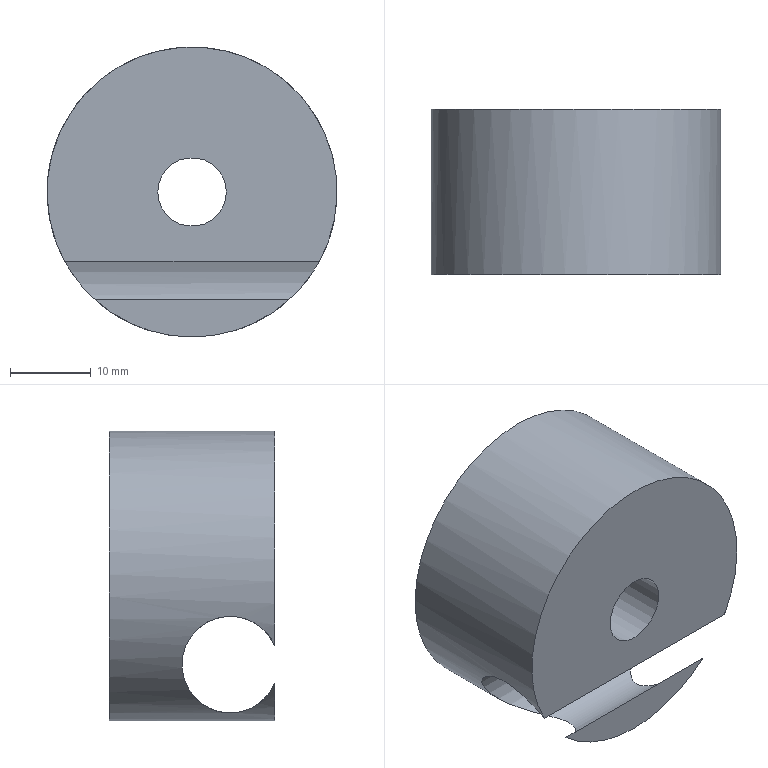Part | STEP file | 冲床-300配套压波_id454_x_t | 1 solid | 8 faces | box 36 x 20.5 x 36 mm | volume 15877 mm3 | cylinder 4 | plane 4 | commonest cylinder face diameters 8.5 x1 12 x1 14 x1 36 x1
STEP:
#1=CARTESIAN_POINT('',(1126.,-87.,-85.));
#2=VERTEX_POINT('',#1);
#3=CARTESIAN_POINT('',(1126.,-87.,-103.));
#4=DIRECTION('',(0.,-1.,0.));
#5=DIRECTION('',(0.,0.,1.));
#6=AXIS2_PLACEMENT_3D('',#3,#4,#5);
#7=CIRCLE('',#6,18.);
#8=EDGE_CURVE('',#2,#2,#7,.T.);
#9=ORIENTED_EDGE('',*,*,#8,.T.);
#10=EDGE_LOOP('',(#9));
#11=FACE_BOUND('',#10,.T.);
#12=CARTESIAN_POINT('',(1141.812,-107.5,-111.602));
#13=VERTEX_POINT('',#12);
#14=CARTESIAN_POINT('',(1110.188,-107.5,-111.602));
#15=VERTEX_POINT('',#14);
#16=CARTESIAN_POINT('',(1126.,-107.5,-103.));
#17=DIRECTION('',(0.,-1.,0.));
#18=DIRECTION('',(1.,0.,0.));
#19=AXIS2_PLACEMENT_3D('',#16,#17,#18);
#20=CIRCLE('',#19,18.);
#21=EDGE_CURVE('',#13,#15,#20,.T.);
#22=ORIENTED_EDGE('',*,*,#21,.F.);
#23=CARTESIAN_POINT('',(1138.021,-107.5,-116.398));
#24=VERTEX_POINT('',#23);
#25=CARTESIAN_POINT('',(1141.812,-107.5,-111.602));
#26=CARTESIAN_POINT('',(1142.553,-106.906,-110.24));
#27=CARTESIAN_POINT('',(1142.98,-105.701,-109.004));
#28=CARTESIAN_POINT('',(1143.354,-102.667,-107.819));
#29=CARTESIAN_POINT('',(1143.342,-100.878,-107.881));
#30=CARTESIAN_POINT('',(1142.876,-97.917,-109.307));
#31=CARTESIAN_POINT('',(1142.38,-96.833,-110.626));
#32=CARTESIAN_POINT('',(1140.814,-95.864,-113.345));
#33=CARTESIAN_POINT('',(1139.756,-95.929,-114.718));
#34=CARTESIAN_POINT('',(1137.484,-96.646,-116.952));
#35=CARTESIAN_POINT('',(1136.238,-97.289,-117.872));
#36=CARTESIAN_POINT('',(1134.415,-98.534,-118.928));
#37=CARTESIAN_POINT('',(1133.8,-99.005,-119.234));
#38=CARTESIAN_POINT('',(1132.684,-100.104,-119.724));
#39=CARTESIAN_POINT('',(1132.126,-100.766,-119.926));
#40=CARTESIAN_POINT('',(1131.796,-102.369,-120.042));
#41=CARTESIAN_POINT('',(1132.18,-103.204,-119.914));
#42=CARTESIAN_POINT('',(1133.181,-104.454,-119.514));
#43=CARTESIAN_POINT('',(1133.782,-104.966,-119.245));
#44=CARTESIAN_POINT('',(1135.59,-106.337,-118.293));
#45=CARTESIAN_POINT('',(1136.839,-107.038,-117.458));
#46=CARTESIAN_POINT('',(1138.021,-107.5,-116.398));
#47=B_SPLINE_CURVE_WITH_KNOTS('',3,(#25,#26,#27,#28,#29,#30,#31,#32,#33,#34,#35,#36,#37,#38,#39,#40,#41,#42,#43,#44,#45,#46),.UNSPECIFIED.,.F.,.F.,(4,2,2,2,2,2,2,2,2,2,4),(0.,0.125,0.25,0.375,0.5,0.625,0.6875,0.75,0.8125,0.875,1.),.UNSPECIFIED.);
#48=EDGE_CURVE('',#13,#24,#47,.T.);
#49=ORIENTED_EDGE('',*,*,#48,.T.);
#50=CARTESIAN_POINT('',(1113.979,-107.5,-116.398));
#51=VERTEX_POINT('',#50);
#52=CARTESIAN_POINT('',(1126.,-107.5,-103.));
#53=DIRECTION('',(0.,-1.,0.));
#54=DIRECTION('',(1.,0.,0.));
#55=AXIS2_PLACEMENT_3D('',#52,#53,#54);
#56=CIRCLE('',#55,18.);
#57=EDGE_CURVE('',#51,#24,#56,.T.);
#58=ORIENTED_EDGE('',*,*,#57,.F.);
#59=CARTESIAN_POINT('',(1113.979,-107.5,-116.398));
#60=CARTESIAN_POINT('',(1115.162,-107.037,-117.459));
#61=CARTESIAN_POINT('',(1116.404,-106.341,-118.29));
#62=CARTESIAN_POINT('',(1118.222,-104.963,-119.247));
#63=CARTESIAN_POINT('',(1118.822,-104.45,-119.516));
#64=CARTESIAN_POINT('',(1119.819,-103.205,-119.914));
#65=CARTESIAN_POINT('',(1120.205,-102.374,-120.043));
#66=CARTESIAN_POINT('',(1119.873,-100.76,-119.926));
#67=CARTESIAN_POINT('',(1119.316,-100.104,-119.724));
#68=CARTESIAN_POINT('',(1118.201,-99.005,-119.234));
#69=CARTESIAN_POINT('',(1117.586,-98.534,-118.928));
#70=CARTESIAN_POINT('',(1115.76,-97.287,-117.87));
#71=CARTESIAN_POINT('',(1114.517,-96.646,-116.953));
#72=CARTESIAN_POINT('',(1112.244,-95.929,-114.718));
#73=CARTESIAN_POINT('',(1111.191,-95.863,-113.353));
#74=CARTESIAN_POINT('',(1109.621,-96.83,-110.63));
#75=CARTESIAN_POINT('',(1109.125,-97.923,-109.309));
#76=CARTESIAN_POINT('',(1108.662,-100.843,-107.893));
#77=CARTESIAN_POINT('',(1108.644,-102.64,-107.812));
#78=CARTESIAN_POINT('',(1109.019,-105.707,-109.004));
#79=CARTESIAN_POINT('',(1109.446,-106.905,-110.238));
#80=CARTESIAN_POINT('',(1110.188,-107.5,-111.602));
#81=B_SPLINE_CURVE_WITH_KNOTS('',3,(#59,#60,#61,#62,#63,#64,#65,#66,#67,#68,#69,#70,#71,#72,#73,#74,#75,#76,#77,#78,#79,#80),.UNSPECIFIED.,.F.,.F.,(4,2,2,2,2,2,2,2,2,2,4),(0.,0.125,0.1875,0.25,0.3125,0.375,0.5,0.625,0.75,0.875,1.),.UNSPECIFIED.);
#82=EDGE_CURVE('',#51,#15,#81,.T.);
#83=ORIENTED_EDGE('',*,*,#82,.T.);
#84=EDGE_LOOP('',(#22,#49,#58,#83));
#85=FACE_BOUND('',#84,.T.);
#86=CARTESIAN_POINT('',(1126.,-87.,-103.));
#87=DIRECTION('',(0.,-1.,0.));
#88=DIRECTION('',(1.,0.,0.));
#89=AXIS2_PLACEMENT_3D('',#86,#87,#88);
#90=CYLINDRICAL_SURFACE('',#89,18.);
#91=ADVANCED_FACE('',(#11,#85),#90,.T.);
#92=CARTESIAN_POINT('',(1130.25,-107.5,-103.));
#93=VERTEX_POINT('',#92);
#94=CARTESIAN_POINT('',(1126.,-107.5,-103.));
#95=DIRECTION('',(0.,-1.,0.));
#96=DIRECTION('',(1.,0.,0.));
#97=AXIS2_PLACEMENT_3D('',#94,#95,#96);
#98=CIRCLE('',#97,4.25);
#99=EDGE_CURVE('',#93,#93,#98,.T.);
#100=ORIENTED_EDGE('',*,*,#99,.F.);
#101=EDGE_LOOP('',(#100));
#102=FACE_BOUND('',#101,.T.);
#103=ORIENTED_EDGE('',*,*,#21,.T.);
#104=CARTESIAN_POINT('',(1172.,-107.5,-111.602));
#105=DIRECTION('',(1.,0.,0.));
#106=VECTOR('',#105,1.);
#107=LINE('',#104,#106);
#108=EDGE_CURVE('',#15,#13,#107,.T.);
#109=ORIENTED_EDGE('',*,*,#108,.T.);
#110=EDGE_LOOP('',(#103,#109));
#111=FACE_BOUND('',#110,.T.);
#112=CARTESIAN_POINT('',(1126.,-107.5,-103.));
#113=DIRECTION('',(0.,-1.,0.));
#114=DIRECTION('',(1.,0.,0.));
#115=AXIS2_PLACEMENT_3D('',#112,#113,#114);
#116=PLANE('',#115);
#117=ADVANCED_FACE('',(#102,#111),#116,.T.);
#118=ORIENTED_EDGE('',*,*,#57,.T.);
#119=CARTESIAN_POINT('',(1172.,-107.5,-116.398));
#120=DIRECTION('',(-1.,0.,0.));
#121=VECTOR('',#120,1.);
#122=LINE('',#119,#121);
#123=EDGE_CURVE('',#24,#51,#122,.T.);
#124=ORIENTED_EDGE('',*,*,#123,.T.);
#125=EDGE_LOOP('',(#118,#124));
#126=FACE_OUTER_BOUND('',#125,.T.);
#127=CARTESIAN_POINT('',(1126.,-107.5,-104.));
#128=DIRECTION('',(0.,-1.,0.));
#129=DIRECTION('',(1.,0.,0.));
#130=AXIS2_PLACEMENT_3D('',#127,#128,#129);
#131=PLANE('',#130);
#132=ADVANCED_FACE('',(#126),#131,.T.);
#133=CARTESIAN_POINT('',(1133.,-87.,-103.));
#134=VERTEX_POINT('',#133);
#135=CARTESIAN_POINT('',(1126.,-87.,-103.));
#136=DIRECTION('',(0.,-1.,0.));
#137=DIRECTION('',(1.,0.,0.));
#138=AXIS2_PLACEMENT_3D('',#135,#136,#137);
#139=CIRCLE('',#138,7.);
#140=EDGE_CURVE('',#134,#134,#139,.T.);
#141=ORIENTED_EDGE('',*,*,#140,.T.);
#142=EDGE_LOOP('',(#141));
#143=FACE_BOUND('',#142,.T.);
#144=ORIENTED_EDGE('',*,*,#8,.F.);
#145=EDGE_LOOP('',(#144));
#146=FACE_BOUND('',#145,.T.);
#147=CARTESIAN_POINT('',(1126.,-87.,-103.));
#148=DIRECTION('',(0.,-1.,0.));
#149=DIRECTION('',(1.,0.,0.));
#150=AXIS2_PLACEMENT_3D('',#147,#148,#149);
#151=PLANE('',#150);
#152=ADVANCED_FACE('',(#143,#146),#151,.F.);
#153=ORIENTED_EDGE('',*,*,#82,.F.);
#154=ORIENTED_EDGE('',*,*,#123,.F.);
#155=ORIENTED_EDGE('',*,*,#48,.F.);
#156=ORIENTED_EDGE('',*,*,#108,.F.);
#157=EDGE_LOOP('',(#153,#154,#155,#156));
#158=FACE_OUTER_BOUND('',#157,.T.);
#159=CARTESIAN_POINT('',(1172.,-102.,-114.));
#160=DIRECTION('',(-1.,0.,0.));
#161=DIRECTION('',(0.,0.,-1.));
#162=AXIS2_PLACEMENT_3D('',#159,#160,#161);
#163=CYLINDRICAL_SURFACE('',#162,6.);
#164=ADVANCED_FACE('',(#158),#163,.F.);
#165=ORIENTED_EDGE('',*,*,#99,.T.);
#166=EDGE_LOOP('',(#165));
#167=FACE_BOUND('',#166,.T.);
#168=CARTESIAN_POINT('',(1130.25,-95.,-103.));
#169=VERTEX_POINT('',#168);
#170=CARTESIAN_POINT('',(1126.,-95.,-103.));
#171=DIRECTION('',(0.,1.,0.));
#172=DIRECTION('',(1.,0.,0.));
#173=AXIS2_PLACEMENT_3D('',#170,#171,#172);
#174=CIRCLE('',#173,4.25);
#175=EDGE_CURVE('',#169,#169,#174,.T.);
#176=ORIENTED_EDGE('',*,*,#175,.T.);
#177=EDGE_LOOP('',(#176));
#178=FACE_BOUND('',#177,.T.);
#179=CARTESIAN_POINT('',(1126.,-127.79,-103.));
#180=DIRECTION('',(0.,-1.,0.));
#181=DIRECTION('',(1.,0.,0.));
#182=AXIS2_PLACEMENT_3D('',#179,#180,#181);
#183=CYLINDRICAL_SURFACE('',#182,4.25);
#184=ADVANCED_FACE('',(#167,#178),#183,.F.);
#185=ORIENTED_EDGE('',*,*,#175,.F.);
#186=EDGE_LOOP('',(#185));
#187=FACE_BOUND('',#186,.T.);
#188=CARTESIAN_POINT('',(1133.,-95.,-103.));
#189=VERTEX_POINT('',#188);
#190=CARTESIAN_POINT('',(1126.,-95.,-103.));
#191=DIRECTION('',(0.,1.,0.));
#192=DIRECTION('',(1.,0.,0.));
#193=AXIS2_PLACEMENT_3D('',#190,#191,#192);
#194=CIRCLE('',#193,7.);
#195=EDGE_CURVE('',#189,#189,#194,.T.);
#196=ORIENTED_EDGE('',*,*,#195,.T.);
#197=EDGE_LOOP('',(#196));
#198=FACE_BOUND('',#197,.T.);
#199=CARTESIAN_POINT('',(1126.,-95.,-103.));
#200=DIRECTION('',(0.,-1.,0.));
#201=DIRECTION('',(1.,0.,0.));
#202=AXIS2_PLACEMENT_3D('',#199,#200,#201);
#203=PLANE('',#202);
#204=ADVANCED_FACE('',(#187,#198),#203,.F.);
#205=ORIENTED_EDGE('',*,*,#195,.F.);
#206=EDGE_LOOP('',(#205));
#207=FACE_BOUND('',#206,.T.);
#208=ORIENTED_EDGE('',*,*,#140,.F.);
#209=EDGE_LOOP('',(#208));
#210=FACE_BOUND('',#209,.T.);
#211=CARTESIAN_POINT('',(1126.,-87.,-103.));
#212=DIRECTION('',(0.,-1.,0.));
#213=DIRECTION('',(1.,0.,0.));
#214=AXIS2_PLACEMENT_3D('',#211,#212,#213);
#215=CYLINDRICAL_SURFACE('',#214,7.);
#216=ADVANCED_FACE('',(#207,#210),#215,.F.);
#217=CLOSED_SHELL('',(#91,#117,#132,#152,#164,#184,#204,#216));
#218=MANIFOLD_SOLID_BREP('',#217);
#219=(LENGTH_UNIT()NAMED_UNIT(*)SI_UNIT(.MILLI.,.METRE.));
#220=UNCERTAINTY_MEASURE_WITH_UNIT(LENGTH_MEASURE(0.0508),#219,'','');
#221=(NAMED_UNIT(*)PLANE_ANGLE_UNIT()SI_UNIT($,.RADIAN.));
#222=PLANE_ANGLE_MEASURE_WITH_UNIT(PLANE_ANGLE_MEASURE(0.01745),#221);
#223=DIMENSIONAL_EXPONENTS(0.,0.,0.,0.,0.,0.,0.);
#224=(CONVERSION_BASED_UNIT('DEGREE',#222)NAMED_UNIT(#223)PLANE_ANGLE_UNIT());
#225=(NAMED_UNIT(*)SI_UNIT($,.STERADIAN.)SOLID_ANGLE_UNIT());
#226=(GEOMETRIC_REPRESENTATION_CONTEXT(3)GLOBAL_UNCERTAINTY_ASSIGNED_CONTEXT((#220))GLOBAL_UNIT_ASSIGNED_CONTEXT((#219,#224,#225))REPRESENTATION_CONTEXT('',''));
#227=ADVANCED_BREP_SHAPE_REPRESENTATION('',(#218),#226);